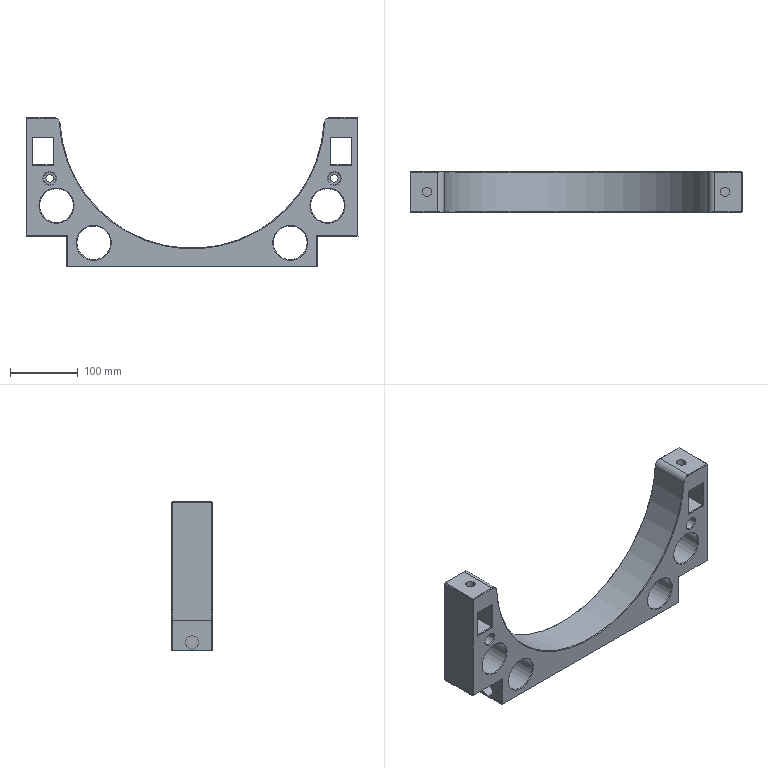Part | NX | features BREP 1 | 1 solid | 130 faces | box 490 x 60 x 220 mm | volume 1895027 mm3 | plane 65 | cylinder 39 | cone 26 | commonest cylinder face diameters 50 x8 20 x6 8.376 x4 11 x4 13.835 x4 18 x4